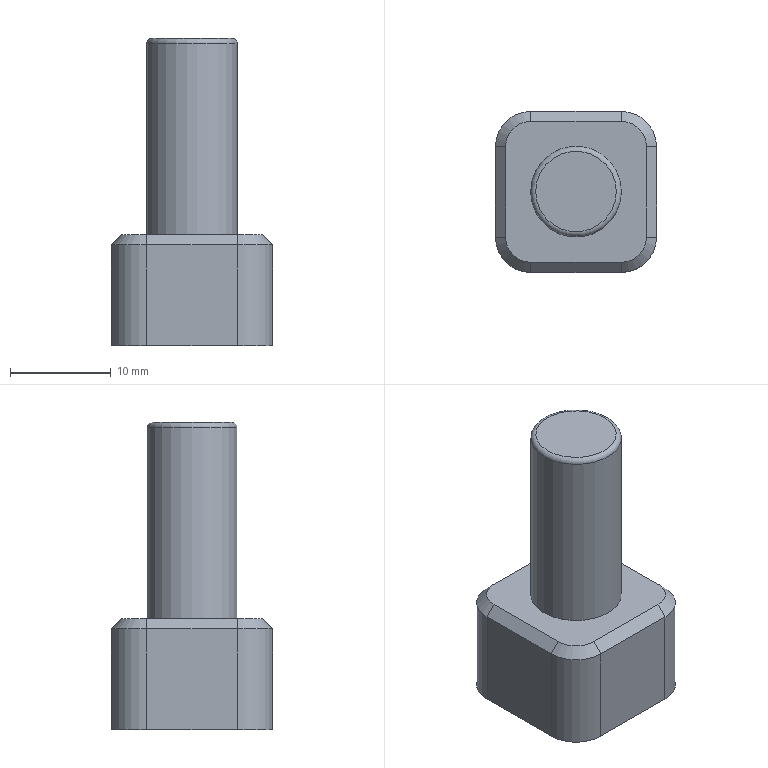CAM job | NX | 3-axis milling | part box 16 x 16 x 30.5 mm | stock box 25 x 25 x 41 mm
Tools:
number,name,description,diameter,corner_radius,flute_length,length,flutes
0,D12-36-D12-75-3T_ROUGH,D12-36-D12-75-3T,12.0,0.0,36.0,75.0,3
0,D12-36-D12-120-3T_FINISH,D12-55-D12-120-3T,12.0,0.0,55.0,120.0,3
0,CHAMFER_D8-90DEG,倒角D8-90度,8.0,0.0,8.0,60.0,2
0,MILL,Milling Tool-5 Parameters,6.0,0.5,50.0,75.0,2
Operations:
program,operation,operation_type,tool,method,geometry_group,spindle_rpm,surface_speed,feed_per_tooth,feed_cut,feed_plunge,cut_length_mm,path_length_mm,cut_time_min,machine_time_min
A1,DYNAMIC_ROUGH,CavityMilling,D12-36-D12-75-3T_ROUGH,METHOD,WORKPIECE_54,6500.0,100.0,0.1178,3000.0,100.0,1229.919,2043.765,0.41,0.4914
A1,FLOOR_WALL,VolumeBased25DMillingOperation,D12-36-D12-120-3T_FINISH,METHOD,WORKPIECE_54,6500.0,245.0,0.0154,300.0,100.0,31.923,131.923,0.1064,0.1164
A1,PLANAR_MILL_COPY,PlanarMilling,D12-36-D12-120-3T_FINISH,METHOD,WORKPIECE_54,6500.0,245.0,0.0154,300.0,100.0,229.854,364.854,0.7662,0.7797
A1,PLANAR_MILL,PlanarMilling,D12-36-D12-120-3T_FINISH,METHOD,WORKPIECE_54,6500.0,245.0,0.0154,300.0,100.0,212.677,370.677,0.7089,0.7247
A1,PLANAR_MILL_COPY_1,PlanarMilling,CHAMFER_D8-90DEG,METHOD,WORKPIECE_54,3000.0,75.0,0.1333,800.0,100.0,87.239,229.239,0.109,0.1232
A1,ZLEVEL_PROFILE_STEEP,ZLevelMilling,MILL,METHOD,WORKPIECE_54,4500.0,84.0,0.2222,2000.0,100.0,929.22,1030.27,0.4646,0.4747
B1,DYNAMIC_ROUGH_COPY,CavityMilling,D12-36-D12-75-3T_ROUGH,METHOD,WORKPIECE_55,6500.0,100.0,0.1178,3000.0,100.0,829.506,868.306,0.2765,0.2804
B1,FLOOR_WALL_1,VolumeBased25DMillingOperation,D12-36-D12-120-3T_FINISH,METHOD,WORKPIECE_55,4500.0,169.0,0.0741,1000.0,100.0,76.177,110.177,0.0762,0.0796
B1,PLANAR_MILL_2,PlanarMilling,CHAMFER_D8-90DEG,METHOD,WORKPIECE_55,4500.0,113.0,0.1111,1000.0,100.0,74.558,113.558,0.0746,0.0785
FIXTURE_1,PLANAR_MILL_1,PlanarMilling,D12-36-D12-75-3T_ROUGH,METHOD,A-G54,4500.0,169.0,0.0593,800.0,100.0,271.35,372.35,0.3392,0.3493